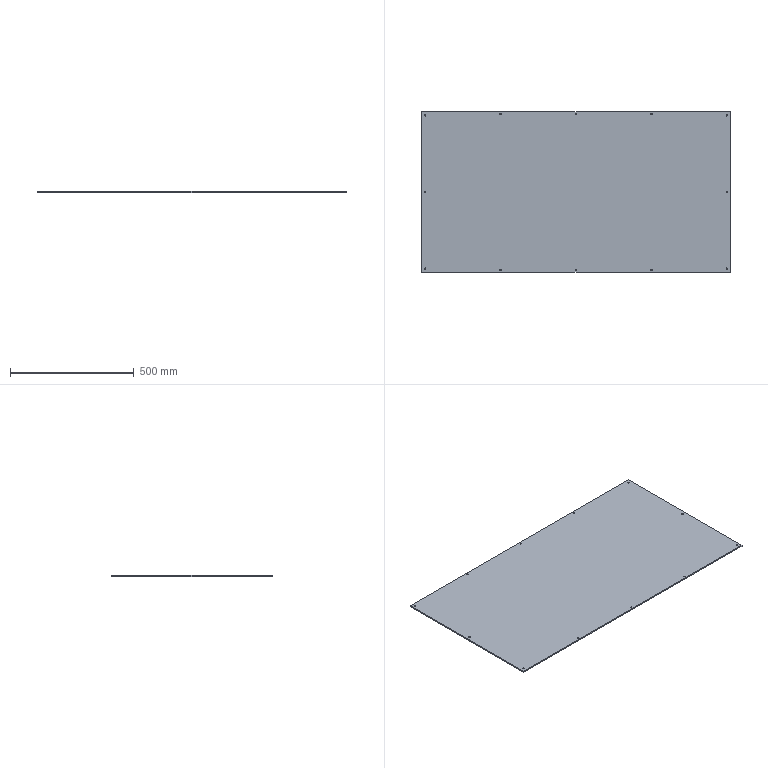Part | SolidWorks | features BaseBody 1 | 1 solid | 30 faces | box 1250 x 650 x 5 mm | volume 4061075 mm3 | cylinder 24 | plane 6 | commonest cylinder face diameters 5.5 x24
STEP:
#1=CARTESIAN_POINT('',(607.25,0.,-2.5));
#2=VERTEX_POINT('',#1);
#3=CARTESIAN_POINT('',(612.75,0.,-2.5));
#4=VERTEX_POINT('',#3);
#5=CARTESIAN_POINT('',(610.,0.,-2.5));
#6=DIRECTION('',(0.,0.,1.));
#7=DIRECTION('',(1.,0.,0.));
#8=AXIS2_PLACEMENT_3D('',#5,#6,#7);
#9=CIRCLE('',#8,2.75);
#10=EDGE_CURVE('',#2,#4,#9,.T.);
#11=ORIENTED_EDGE('',*,*,#10,.F.);
#12=CARTESIAN_POINT('',(607.25,0.,2.5));
#13=VERTEX_POINT('',#12);
#14=CARTESIAN_POINT('',(607.25,0.,2.5));
#15=DIRECTION('',(0.,0.,1.));
#16=VECTOR('',#15,1000.);
#17=LINE('',#14,#16);
#18=EDGE_CURVE('',#2,#13,#17,.T.);
#19=ORIENTED_EDGE('',*,*,#18,.T.);
#20=CARTESIAN_POINT('',(612.75,0.,2.5));
#21=VERTEX_POINT('',#20);
#22=CARTESIAN_POINT('',(610.,0.,2.5));
#23=DIRECTION('',(0.,0.,1.));
#24=DIRECTION('',(1.,0.,0.));
#25=AXIS2_PLACEMENT_3D('',#22,#23,#24);
#26=CIRCLE('',#25,2.75);
#27=EDGE_CURVE('',#13,#21,#26,.T.);
#28=ORIENTED_EDGE('',*,*,#27,.T.);
#29=CARTESIAN_POINT('',(612.75,0.,2.5));
#30=DIRECTION('',(0.,0.,1.));
#31=VECTOR('',#30,1000.);
#32=LINE('',#29,#31);
#33=EDGE_CURVE('',#4,#21,#32,.T.);
#34=ORIENTED_EDGE('',*,*,#33,.F.);
#35=EDGE_LOOP('',(#11,#19,#28,#34));
#36=FACE_OUTER_BOUND('',#35,.T.);
#37=CARTESIAN_POINT('',(610.,0.,2.5));
#38=DIRECTION('',(0.,0.,1.));
#39=DIRECTION('',(1.,0.,0.));
#40=AXIS2_PLACEMENT_3D('',#37,#38,#39);
#41=CYLINDRICAL_SURFACE('',#40,2.75);
#42=ADVANCED_FACE('',(#36),#41,.F.);
#43=CARTESIAN_POINT('',(607.25,-310.,-2.5));
#44=VERTEX_POINT('',#43);
#45=CARTESIAN_POINT('',(612.75,-310.,-2.5));
#46=VERTEX_POINT('',#45);
#47=CARTESIAN_POINT('',(610.,-310.,-2.5));
#48=DIRECTION('',(0.,0.,1.));
#49=DIRECTION('',(1.,0.,0.));
#50=AXIS2_PLACEMENT_3D('',#47,#48,#49);
#51=CIRCLE('',#50,2.75);
#52=EDGE_CURVE('',#44,#46,#51,.T.);
#53=ORIENTED_EDGE('',*,*,#52,.F.);
#54=CARTESIAN_POINT('',(607.25,-310.,2.5));
#55=VERTEX_POINT('',#54);
#56=CARTESIAN_POINT('',(607.25,-310.,2.5));
#57=DIRECTION('',(0.,0.,1.));
#58=VECTOR('',#57,1000.);
#59=LINE('',#56,#58);
#60=EDGE_CURVE('',#44,#55,#59,.T.);
#61=ORIENTED_EDGE('',*,*,#60,.T.);
#62=CARTESIAN_POINT('',(612.75,-310.,2.5));
#63=VERTEX_POINT('',#62);
#64=CARTESIAN_POINT('',(610.,-310.,2.5));
#65=DIRECTION('',(0.,0.,1.));
#66=DIRECTION('',(1.,0.,0.));
#67=AXIS2_PLACEMENT_3D('',#64,#65,#66);
#68=CIRCLE('',#67,2.75);
#69=EDGE_CURVE('',#55,#63,#68,.T.);
#70=ORIENTED_EDGE('',*,*,#69,.T.);
#71=CARTESIAN_POINT('',(612.75,-310.,2.5));
#72=DIRECTION('',(0.,0.,1.));
#73=VECTOR('',#72,1000.);
#74=LINE('',#71,#73);
#75=EDGE_CURVE('',#46,#63,#74,.T.);
#76=ORIENTED_EDGE('',*,*,#75,.F.);
#77=EDGE_LOOP('',(#53,#61,#70,#76));
#78=FACE_OUTER_BOUND('',#77,.T.);
#79=CARTESIAN_POINT('',(610.,-310.,2.5));
#80=DIRECTION('',(0.,0.,1.));
#81=DIRECTION('',(1.,0.,0.));
#82=AXIS2_PLACEMENT_3D('',#79,#80,#81);
#83=CYLINDRICAL_SURFACE('',#82,2.75);
#84=ADVANCED_FACE('',(#78),#83,.F.);
#85=CARTESIAN_POINT('',(607.25,310.,-2.5));
#86=VERTEX_POINT('',#85);
#87=CARTESIAN_POINT('',(612.75,310.,-2.5));
#88=VERTEX_POINT('',#87);
#89=CARTESIAN_POINT('',(610.,310.,-2.5));
#90=DIRECTION('',(0.,0.,1.));
#91=DIRECTION('',(1.,0.,0.));
#92=AXIS2_PLACEMENT_3D('',#89,#90,#91);
#93=CIRCLE('',#92,2.75);
#94=EDGE_CURVE('',#86,#88,#93,.T.);
#95=ORIENTED_EDGE('',*,*,#94,.F.);
#96=CARTESIAN_POINT('',(607.25,310.,2.5));
#97=VERTEX_POINT('',#96);
#98=CARTESIAN_POINT('',(607.25,310.,2.5));
#99=DIRECTION('',(0.,0.,1.));
#100=VECTOR('',#99,1000.);
#101=LINE('',#98,#100);
#102=EDGE_CURVE('',#86,#97,#101,.T.);
#103=ORIENTED_EDGE('',*,*,#102,.T.);
#104=CARTESIAN_POINT('',(612.75,310.,2.5));
#105=VERTEX_POINT('',#104);
#106=CARTESIAN_POINT('',(610.,310.,2.5));
#107=DIRECTION('',(0.,0.,1.));
#108=DIRECTION('',(1.,0.,0.));
#109=AXIS2_PLACEMENT_3D('',#106,#107,#108);
#110=CIRCLE('',#109,2.75);
#111=EDGE_CURVE('',#97,#105,#110,.T.);
#112=ORIENTED_EDGE('',*,*,#111,.T.);
#113=CARTESIAN_POINT('',(612.75,310.,2.5));
#114=DIRECTION('',(0.,0.,1.));
#115=VECTOR('',#114,1000.);
#116=LINE('',#113,#115);
#117=EDGE_CURVE('',#88,#105,#116,.T.);
#118=ORIENTED_EDGE('',*,*,#117,.F.);
#119=EDGE_LOOP('',(#95,#103,#112,#118));
#120=FACE_OUTER_BOUND('',#119,.T.);
#121=CARTESIAN_POINT('',(610.,310.,2.5));
#122=DIRECTION('',(0.,0.,1.));
#123=DIRECTION('',(1.,0.,0.));
#124=AXIS2_PLACEMENT_3D('',#121,#122,#123);
#125=CYLINDRICAL_SURFACE('',#124,2.75);
#126=ADVANCED_FACE('',(#120),#125,.F.);
#127=CARTESIAN_POINT('',(302.25,-316.,-2.5));
#128=VERTEX_POINT('',#127);
#129=CARTESIAN_POINT('',(307.75,-316.,-2.5));
#130=VERTEX_POINT('',#129);
#131=CARTESIAN_POINT('',(305.,-316.,-2.5));
#132=DIRECTION('',(0.,0.,1.));
#133=DIRECTION('',(1.,0.,0.));
#134=AXIS2_PLACEMENT_3D('',#131,#132,#133);
#135=CIRCLE('',#134,2.75);
#136=EDGE_CURVE('',#128,#130,#135,.T.);
#137=ORIENTED_EDGE('',*,*,#136,.F.);
#138=CARTESIAN_POINT('',(302.25,-316.,2.5));
#139=VERTEX_POINT('',#138);
#140=CARTESIAN_POINT('',(302.25,-316.,2.5));
#141=DIRECTION('',(0.,0.,1.));
#142=VECTOR('',#141,1000.);
#143=LINE('',#140,#142);
#144=EDGE_CURVE('',#128,#139,#143,.T.);
#145=ORIENTED_EDGE('',*,*,#144,.T.);
#146=CARTESIAN_POINT('',(307.75,-316.,2.5));
#147=VERTEX_POINT('',#146);
#148=CARTESIAN_POINT('',(305.,-316.,2.5));
#149=DIRECTION('',(0.,0.,1.));
#150=DIRECTION('',(1.,0.,0.));
#151=AXIS2_PLACEMENT_3D('',#148,#149,#150);
#152=CIRCLE('',#151,2.75);
#153=EDGE_CURVE('',#139,#147,#152,.T.);
#154=ORIENTED_EDGE('',*,*,#153,.T.);
#155=CARTESIAN_POINT('',(307.75,-316.,2.5));
#156=DIRECTION('',(0.,0.,1.));
#157=VECTOR('',#156,1000.);
#158=LINE('',#155,#157);
#159=EDGE_CURVE('',#130,#147,#158,.T.);
#160=ORIENTED_EDGE('',*,*,#159,.F.);
#161=EDGE_LOOP('',(#137,#145,#154,#160));
#162=FACE_OUTER_BOUND('',#161,.T.);
#163=CARTESIAN_POINT('',(305.,-316.,2.5));
#164=DIRECTION('',(0.,0.,1.));
#165=DIRECTION('',(1.,0.,0.));
#166=AXIS2_PLACEMENT_3D('',#163,#164,#165);
#167=CYLINDRICAL_SURFACE('',#166,2.75);
#168=ADVANCED_FACE('',(#162),#167,.F.);
#169=CARTESIAN_POINT('',(302.25,316.,-2.5));
#170=VERTEX_POINT('',#169);
#171=CARTESIAN_POINT('',(307.75,316.,-2.5));
#172=VERTEX_POINT('',#171);
#173=CARTESIAN_POINT('',(305.,316.,-2.5));
#174=DIRECTION('',(0.,0.,1.));
#175=DIRECTION('',(1.,0.,0.));
#176=AXIS2_PLACEMENT_3D('',#173,#174,#175);
#177=CIRCLE('',#176,2.75);
#178=EDGE_CURVE('',#170,#172,#177,.T.);
#179=ORIENTED_EDGE('',*,*,#178,.F.);
#180=CARTESIAN_POINT('',(302.25,316.,2.5));
#181=VERTEX_POINT('',#180);
#182=CARTESIAN_POINT('',(302.25,316.,2.5));
#183=DIRECTION('',(0.,0.,1.));
#184=VECTOR('',#183,1000.);
#185=LINE('',#182,#184);
#186=EDGE_CURVE('',#170,#181,#185,.T.);
#187=ORIENTED_EDGE('',*,*,#186,.T.);
#188=CARTESIAN_POINT('',(307.75,316.,2.5));
#189=VERTEX_POINT('',#188);
#190=CARTESIAN_POINT('',(305.,316.,2.5));
#191=DIRECTION('',(0.,0.,1.));
#192=DIRECTION('',(1.,0.,0.));
#193=AXIS2_PLACEMENT_3D('',#190,#191,#192);
#194=CIRCLE('',#193,2.75);
#195=EDGE_CURVE('',#181,#189,#194,.T.);
#196=ORIENTED_EDGE('',*,*,#195,.T.);
#197=CARTESIAN_POINT('',(307.75,316.,2.5));
#198=DIRECTION('',(0.,0.,1.));
#199=VECTOR('',#198,1000.);
#200=LINE('',#197,#199);
#201=EDGE_CURVE('',#172,#189,#200,.T.);
#202=ORIENTED_EDGE('',*,*,#201,.F.);
#203=EDGE_LOOP('',(#179,#187,#196,#202));
#204=FACE_OUTER_BOUND('',#203,.T.);
#205=CARTESIAN_POINT('',(305.,316.,2.5));
#206=DIRECTION('',(0.,0.,1.));
#207=DIRECTION('',(1.,0.,0.));
#208=AXIS2_PLACEMENT_3D('',#205,#206,#207);
#209=CYLINDRICAL_SURFACE('',#208,2.75);
#210=ADVANCED_FACE('',(#204),#209,.F.);
#211=CARTESIAN_POINT('',(-2.75,-316.,-2.5));
#212=VERTEX_POINT('',#211);
#213=CARTESIAN_POINT('',(2.75,-316.,-2.5));
#214=VERTEX_POINT('',#213);
#215=CARTESIAN_POINT('',(0.,-316.,-2.5));
#216=DIRECTION('',(0.,0.,1.));
#217=DIRECTION('',(1.,0.,0.));
#218=AXIS2_PLACEMENT_3D('',#215,#216,#217);
#219=CIRCLE('',#218,2.75);
#220=EDGE_CURVE('',#212,#214,#219,.T.);
#221=ORIENTED_EDGE('',*,*,#220,.F.);
#222=CARTESIAN_POINT('',(-2.75,-316.,2.5));
#223=VERTEX_POINT('',#222);
#224=CARTESIAN_POINT('',(-2.75,-316.,2.5));
#225=DIRECTION('',(0.,0.,1.));
#226=VECTOR('',#225,1000.);
#227=LINE('',#224,#226);
#228=EDGE_CURVE('',#212,#223,#227,.T.);
#229=ORIENTED_EDGE('',*,*,#228,.T.);
#230=CARTESIAN_POINT('',(2.75,-316.,2.5));
#231=VERTEX_POINT('',#230);
#232=CARTESIAN_POINT('',(0.,-316.,2.5));
#233=DIRECTION('',(0.,0.,1.));
#234=DIRECTION('',(1.,0.,0.));
#235=AXIS2_PLACEMENT_3D('',#232,#233,#234);
#236=CIRCLE('',#235,2.75);
#237=EDGE_CURVE('',#223,#231,#236,.T.);
#238=ORIENTED_EDGE('',*,*,#237,.T.);
#239=CARTESIAN_POINT('',(2.75,-316.,2.5));
#240=DIRECTION('',(0.,0.,1.));
#241=VECTOR('',#240,1000.);
#242=LINE('',#239,#241);
#243=EDGE_CURVE('',#214,#231,#242,.T.);
#244=ORIENTED_EDGE('',*,*,#243,.F.);
#245=EDGE_LOOP('',(#221,#229,#238,#244));
#246=FACE_OUTER_BOUND('',#245,.T.);
#247=CARTESIAN_POINT('',(0.,-316.,2.5));
#248=DIRECTION('',(0.,0.,1.));
#249=DIRECTION('',(1.,0.,0.));
#250=AXIS2_PLACEMENT_3D('',#247,#248,#249);
#251=CYLINDRICAL_SURFACE('',#250,2.75);
#252=ADVANCED_FACE('',(#246),#251,.F.);
#253=CARTESIAN_POINT('',(-2.75,316.,-2.5));
#254=VERTEX_POINT('',#253);
#255=CARTESIAN_POINT('',(2.75,316.,-2.5));
#256=VERTEX_POINT('',#255);
#257=CARTESIAN_POINT('',(0.,316.,-2.5));
#258=DIRECTION('',(0.,0.,1.));
#259=DIRECTION('',(1.,0.,0.));
#260=AXIS2_PLACEMENT_3D('',#257,#258,#259);
#261=CIRCLE('',#260,2.75);
#262=EDGE_CURVE('',#254,#256,#261,.T.);
#263=ORIENTED_EDGE('',*,*,#262,.F.);
#264=CARTESIAN_POINT('',(-2.75,316.,2.5));
#265=VERTEX_POINT('',#264);
#266=CARTESIAN_POINT('',(-2.75,316.,2.5));
#267=DIRECTION('',(0.,0.,1.));
#268=VECTOR('',#267,1000.);
#269=LINE('',#266,#268);
#270=EDGE_CURVE('',#254,#265,#269,.T.);
#271=ORIENTED_EDGE('',*,*,#270,.T.);
#272=CARTESIAN_POINT('',(2.75,316.,2.5));
#273=VERTEX_POINT('',#272);
#274=CARTESIAN_POINT('',(0.,316.,2.5));
#275=DIRECTION('',(0.,0.,1.));
#276=DIRECTION('',(1.,0.,0.));
#277=AXIS2_PLACEMENT_3D('',#274,#275,#276);
#278=CIRCLE('',#277,2.75);
#279=EDGE_CURVE('',#265,#273,#278,.T.);
#280=ORIENTED_EDGE('',*,*,#279,.T.);
#281=CARTESIAN_POINT('',(2.75,316.,2.5));
#282=DIRECTION('',(0.,0.,1.));
#283=VECTOR('',#282,1000.);
#284=LINE('',#281,#283);
#285=EDGE_CURVE('',#256,#273,#284,.T.);
#286=ORIENTED_EDGE('',*,*,#285,.F.);
#287=EDGE_LOOP('',(#263,#271,#280,#286));
#288=FACE_OUTER_BOUND('',#287,.T.);
#289=CARTESIAN_POINT('',(0.,316.,2.5));
#290=DIRECTION('',(0.,0.,1.));
#291=DIRECTION('',(1.,0.,0.));
#292=AXIS2_PLACEMENT_3D('',#289,#290,#291);
#293=CYLINDRICAL_SURFACE('',#292,2.75);
#294=ADVANCED_FACE('',(#288),#293,.F.);
#295=CARTESIAN_POINT('',(-307.75,-316.,-2.5));
#296=VERTEX_POINT('',#295);
#297=CARTESIAN_POINT('',(-302.25,-316.,-2.5));
#298=VERTEX_POINT('',#297);
#299=CARTESIAN_POINT('',(-305.,-316.,-2.5));
#300=DIRECTION('',(0.,0.,1.));
#301=DIRECTION('',(1.,0.,0.));
#302=AXIS2_PLACEMENT_3D('',#299,#300,#301);
#303=CIRCLE('',#302,2.75);
#304=EDGE_CURVE('',#296,#298,#303,.T.);
#305=ORIENTED_EDGE('',*,*,#304,.F.);
#306=CARTESIAN_POINT('',(-307.75,-316.,2.5));
#307=VERTEX_POINT('',#306);
#308=CARTESIAN_POINT('',(-307.75,-316.,2.5));
#309=DIRECTION('',(0.,0.,1.));
#310=VECTOR('',#309,1000.);
#311=LINE('',#308,#310);
#312=EDGE_CURVE('',#296,#307,#311,.T.);
#313=ORIENTED_EDGE('',*,*,#312,.T.);
#314=CARTESIAN_POINT('',(-302.25,-316.,2.5));
#315=VERTEX_POINT('',#314);
#316=CARTESIAN_POINT('',(-305.,-316.,2.5));
#317=DIRECTION('',(0.,0.,1.));
#318=DIRECTION('',(1.,0.,0.));
#319=AXIS2_PLACEMENT_3D('',#316,#317,#318);
#320=CIRCLE('',#319,2.75);
#321=EDGE_CURVE('',#307,#315,#320,.T.);
#322=ORIENTED_EDGE('',*,*,#321,.T.);
#323=CARTESIAN_POINT('',(-302.25,-316.,2.5));
#324=DIRECTION('',(0.,0.,1.));
#325=VECTOR('',#324,1000.);
#326=LINE('',#323,#325);
#327=EDGE_CURVE('',#298,#315,#326,.T.);
#328=ORIENTED_EDGE('',*,*,#327,.F.);
#329=EDGE_LOOP('',(#305,#313,#322,#328));
#330=FACE_OUTER_BOUND('',#329,.T.);
#331=CARTESIAN_POINT('',(-305.,-316.,2.5));
#332=DIRECTION('',(0.,0.,1.));
#333=DIRECTION('',(1.,0.,0.));
#334=AXIS2_PLACEMENT_3D('',#331,#332,#333);
#335=CYLINDRICAL_SURFACE('',#334,2.75);
#336=ADVANCED_FACE('',(#330),#335,.F.);
#337=CARTESIAN_POINT('',(-307.75,316.,-2.5));
#338=VERTEX_POINT('',#337);
#339=CARTESIAN_POINT('',(-302.25,316.,-2.5));
#340=VERTEX_POINT('',#339);
#341=CARTESIAN_POINT('',(-305.,316.,-2.5));
#342=DIRECTION('',(0.,0.,1.));
#343=DIRECTION('',(1.,0.,0.));
#344=AXIS2_PLACEMENT_3D('',#341,#342,#343);
#345=CIRCLE('',#344,2.75);
#346=EDGE_CURVE('',#338,#340,#345,.T.);
#347=ORIENTED_EDGE('',*,*,#346,.F.);
#348=CARTESIAN_POINT('',(-307.75,316.,2.5));
#349=VERTEX_POINT('',#348);
#350=CARTESIAN_POINT('',(-307.75,316.,2.5));
#351=DIRECTION('',(0.,0.,1.));
#352=VECTOR('',#351,1000.);
#353=LINE('',#350,#352);
#354=EDGE_CURVE('',#338,#349,#353,.T.);
#355=ORIENTED_EDGE('',*,*,#354,.T.);
#356=CARTESIAN_POINT('',(-302.25,316.,2.5));
#357=VERTEX_POINT('',#356);
#358=CARTESIAN_POINT('',(-305.,316.,2.5));
#359=DIRECTION('',(0.,0.,1.));
#360=DIRECTION('',(1.,0.,0.));
#361=AXIS2_PLACEMENT_3D('',#358,#359,#360);
#362=CIRCLE('',#361,2.75);
#363=EDGE_CURVE('',#349,#357,#362,.T.);
#364=ORIENTED_EDGE('',*,*,#363,.T.);
#365=CARTESIAN_POINT('',(-302.25,316.,2.5));
#366=DIRECTION('',(0.,0.,1.));
#367=VECTOR('',#366,1000.);
#368=LINE('',#365,#367);
#369=EDGE_CURVE('',#340,#357,#368,.T.);
#370=ORIENTED_EDGE('',*,*,#369,.F.);
#371=EDGE_LOOP('',(#347,#355,#364,#370));
#372=FACE_OUTER_BOUND('',#371,.T.);
#373=CARTESIAN_POINT('',(-305.,316.,2.5));
#374=DIRECTION('',(0.,0.,1.));
#375=DIRECTION('',(1.,0.,0.));
#376=AXIS2_PLACEMENT_3D('',#373,#374,#375);
#377=CYLINDRICAL_SURFACE('',#376,2.75);
#378=ADVANCED_FACE('',(#372),#377,.F.);
#379=CARTESIAN_POINT('',(-612.75,-310.,-2.5));
#380=VERTEX_POINT('',#379);
#381=CARTESIAN_POINT('',(-607.25,-310.,-2.5));
#382=VERTEX_POINT('',#381);
#383=CARTESIAN_POINT('',(-610.,-310.,-2.5));
#384=DIRECTION('',(0.,0.,1.));
#385=DIRECTION('',(1.,0.,0.));
#386=AXIS2_PLACEMENT_3D('',#383,#384,#385);
#387=CIRCLE('',#386,2.75);
#388=EDGE_CURVE('',#380,#382,#387,.T.);
#389=ORIENTED_EDGE('',*,*,#388,.F.);
#390=CARTESIAN_POINT('',(-612.75,-310.,2.5));
#391=VERTEX_POINT('',#390);
#392=CARTESIAN_POINT('',(-612.75,-310.,2.5));
#393=DIRECTION('',(0.,0.,1.));
#394=VECTOR('',#393,1000.);
#395=LINE('',#392,#394);
#396=EDGE_CURVE('',#380,#391,#395,.T.);
#397=ORIENTED_EDGE('',*,*,#396,.T.);
#398=CARTESIAN_POINT('',(-607.25,-310.,2.5));
#399=VERTEX_POINT('',#398);
#400=CARTESIAN_POINT('',(-610.,-310.,2.5));
#401=DIRECTION('',(0.,0.,1.));
#402=DIRECTION('',(1.,0.,0.));
#403=AXIS2_PLACEMENT_3D('',#400,#401,#402);
#404=CIRCLE('',#403,2.75);
#405=EDGE_CURVE('',#391,#399,#404,.T.);
#406=ORIENTED_EDGE('',*,*,#405,.T.);
#407=CARTESIAN_POINT('',(-607.25,-310.,2.5));
#408=DIRECTION('',(0.,0.,1.));
#409=VECTOR('',#408,1000.);
#410=LINE('',#407,#409);
#411=EDGE_CURVE('',#382,#399,#410,.T.);
#412=ORIENTED_EDGE('',*,*,#411,.F.);
#413=EDGE_LOOP('',(#389,#397,#406,#412));
#414=FACE_OUTER_BOUND('',#413,.T.);
#415=CARTESIAN_POINT('',(-610.,-310.,2.5));
#416=DIRECTION('',(0.,0.,1.));
#417=DIRECTION('',(1.,0.,0.));
#418=AXIS2_PLACEMENT_3D('',#415,#416,#417);
#419=CYLINDRICAL_SURFACE('',#418,2.75);
#420=ADVANCED_FACE('',(#414),#419,.F.);
#421=CARTESIAN_POINT('',(-612.75,0.,-2.5));
#422=VERTEX_POINT('',#421);
#423=CARTESIAN_POINT('',(-607.25,0.,-2.5));
#424=VERTEX_POINT('',#423);
#425=CARTESIAN_POINT('',(-610.,0.,-2.5));
#426=DIRECTION('',(0.,0.,1.));
#427=DIRECTION('',(1.,0.,0.));
#428=AXIS2_PLACEMENT_3D('',#425,#426,#427);
#429=CIRCLE('',#428,2.75);
#430=EDGE_CURVE('',#422,#424,#429,.T.);
#431=ORIENTED_EDGE('',*,*,#430,.F.);
#432=CARTESIAN_POINT('',(-612.75,0.,2.5));
#433=VERTEX_POINT('',#432);
#434=CARTESIAN_POINT('',(-612.75,0.,2.5));
#435=DIRECTION('',(0.,0.,1.));
#436=VECTOR('',#435,1000.);
#437=LINE('',#434,#436);
#438=EDGE_CURVE('',#422,#433,#437,.T.);
#439=ORIENTED_EDGE('',*,*,#438,.T.);
#440=CARTESIAN_POINT('',(-607.25,0.,2.5));
#441=VERTEX_POINT('',#440);
#442=CARTESIAN_POINT('',(-610.,0.,2.5));
#443=DIRECTION('',(0.,0.,1.));
#444=DIRECTION('',(1.,0.,0.));
#445=AXIS2_PLACEMENT_3D('',#442,#443,#444);
#446=CIRCLE('',#445,2.75);
#447=EDGE_CURVE('',#433,#441,#446,.T.);
#448=ORIENTED_EDGE('',*,*,#447,.T.);
#449=CARTESIAN_POINT('',(-607.25,0.,2.5));
#450=DIRECTION('',(0.,0.,1.));
#451=VECTOR('',#450,1000.);
#452=LINE('',#449,#451);
#453=EDGE_CURVE('',#424,#441,#452,.T.);
#454=ORIENTED_EDGE('',*,*,#453,.F.);
#455=EDGE_LOOP('',(#431,#439,#448,#454));
#456=FACE_OUTER_BOUND('',#455,.T.);
#457=CARTESIAN_POINT('',(-610.,0.,2.5));
#458=DIRECTION('',(0.,0.,1.));
#459=DIRECTION('',(1.,0.,0.));
#460=AXIS2_PLACEMENT_3D('',#457,#458,#459);
#461=CYLINDRICAL_SURFACE('',#460,2.75);
#462=ADVANCED_FACE('',(#456),#461,.F.);
#463=CARTESIAN_POINT('',(-612.75,310.,-2.5));
#464=VERTEX_POINT('',#463);
#465=CARTESIAN_POINT('',(-607.25,310.,-2.5));
#466=VERTEX_POINT('',#465);
#467=CARTESIAN_POINT('',(-610.,310.,-2.5));
#468=DIRECTION('',(0.,0.,1.));
#469=DIRECTION('',(1.,0.,0.));
#470=AXIS2_PLACEMENT_3D('',#467,#468,#469);
#471=CIRCLE('',#470,2.75);
#472=EDGE_CURVE('',#464,#466,#471,.T.);
#473=ORIENTED_EDGE('',*,*,#472,.F.);
#474=CARTESIAN_POINT('',(-612.75,310.,2.5));
#475=VERTEX_POINT('',#474);
#476=CARTESIAN_POINT('',(-612.75,310.,2.5));
#477=DIRECTION('',(0.,0.,1.));
#478=VECTOR('',#477,1000.);
#479=LINE('',#476,#478);
#480=EDGE_CURVE('',#464,#475,#479,.T.);
#481=ORIENTED_EDGE('',*,*,#480,.T.);
#482=CARTESIAN_POINT('',(-607.25,310.,2.5));
#483=VERTEX_POINT('',#482);
#484=CARTESIAN_POINT('',(-610.,310.,2.5));
#485=DIRECTION('',(0.,0.,1.));
#486=DIRECTION('',(1.,0.,0.));
#487=AXIS2_PLACEMENT_3D('',#484,#485,#486);
#488=CIRCLE('',#487,2.75);
#489=EDGE_CURVE('',#475,#483,#488,.T.);
#490=ORIENTED_EDGE('',*,*,#489,.T.);
#491=CARTESIAN_POINT('',(-607.25,310.,2.5));
#492=DIRECTION('',(0.,0.,1.));
#493=VECTOR('',#492,1000.);
#494=LINE('',#491,#493);
#495=EDGE_CURVE('',#466,#483,#494,.T.);
#496=ORIENTED_EDGE('',*,*,#495,.F.);
#497=EDGE_LOOP('',(#473,#481,#490,#496));
#498=FACE_OUTER_BOUND('',#497,.T.);
#499=CARTESIAN_POINT('',(-610.,310.,2.5));
#500=DIRECTION('',(0.,0.,1.));
#501=DIRECTION('',(1.,0.,0.));
#502=AXIS2_PLACEMENT_3D('',#499,#500,#501);
#503=CYLINDRICAL_SURFACE('',#502,2.75);
#504=ADVANCED_FACE('',(#498),#503,.F.);
#505=CARTESIAN_POINT('',(-610.,310.,-2.5));
#506=DIRECTION('',(0.,0.,1.));
#507=DIRECTION('',(1.,0.,0.));
#508=AXIS2_PLACEMENT_3D('',#505,#506,#507);
#509=CIRCLE('',#508,2.75);
#510=EDGE_CURVE('',#466,#464,#509,.T.);
#511=ORIENTED_EDGE('',*,*,#510,.T.);
#512=ORIENTED_EDGE('',*,*,#472,.T.);
#513=EDGE_LOOP('',(#511,#512));
#514=FACE_BOUND('',#513,.T.);
#515=CARTESIAN_POINT('',(-610.,0.,-2.5));
#516=DIRECTION('',(0.,0.,1.));
#517=DIRECTION('',(1.,0.,0.));
#518=AXIS2_PLACEMENT_3D('',#515,#516,#517);
#519=CIRCLE('',#518,2.75);
#520=EDGE_CURVE('',#424,#422,#519,.T.);
#521=ORIENTED_EDGE('',*,*,#520,.T.);
#522=ORIENTED_EDGE('',*,*,#430,.T.);
#523=EDGE_LOOP('',(#521,#522));
#524=FACE_BOUND('',#523,.T.);
#525=CARTESIAN_POINT('',(-610.,-310.,-2.5));
#526=DIRECTION('',(0.,0.,1.));
#527=DIRECTION('',(1.,0.,0.));
#528=AXIS2_PLACEMENT_3D('',#525,#526,#527);
#529=CIRCLE('',#528,2.75);
#530=EDGE_CURVE('',#382,#380,#529,.T.);
#531=ORIENTED_EDGE('',*,*,#530,.T.);
#532=ORIENTED_EDGE('',*,*,#388,.T.);
#533=EDGE_LOOP('',(#531,#532));
#534=FACE_BOUND('',#533,.T.);
#535=CARTESIAN_POINT('',(-305.,316.,-2.5));
#536=DIRECTION('',(0.,0.,1.));
#537=DIRECTION('',(1.,0.,0.));
#538=AXIS2_PLACEMENT_3D('',#535,#536,#537);
#539=CIRCLE('',#538,2.75);
#540=EDGE_CURVE('',#340,#338,#539,.T.);
#541=ORIENTED_EDGE('',*,*,#540,.T.);
#542=ORIENTED_EDGE('',*,*,#346,.T.);
#543=EDGE_LOOP('',(#541,#542));
#544=FACE_BOUND('',#543,.T.);
#545=CARTESIAN_POINT('',(-305.,-316.,-2.5));
#546=DIRECTION('',(0.,0.,1.));
#547=DIRECTION('',(1.,0.,0.));
#548=AXIS2_PLACEMENT_3D('',#545,#546,#547);
#549=CIRCLE('',#548,2.75);
#550=EDGE_CURVE('',#298,#296,#549,.T.);
#551=ORIENTED_EDGE('',*,*,#550,.T.);
#552=ORIENTED_EDGE('',*,*,#304,.T.);
#553=EDGE_LOOP('',(#551,#552));
#554=FACE_BOUND('',#553,.T.);
#555=CARTESIAN_POINT('',(0.,316.,-2.5));
#556=DIRECTION('',(0.,0.,1.));
#557=DIRECTION('',(1.,0.,0.));
#558=AXIS2_PLACEMENT_3D('',#555,#556,#557);
#559=CIRCLE('',#558,2.75);
#560=EDGE_CURVE('',#256,#254,#559,.T.);
#561=ORIENTED_EDGE('',*,*,#560,.T.);
#562=ORIENTED_EDGE('',*,*,#262,.T.);
#563=EDGE_LOOP('',(#561,#562));
#564=FACE_BOUND('',#563,.T.);
#565=CARTESIAN_POINT('',(0.,-316.,-2.5));
#566=DIRECTION('',(0.,0.,1.));
#567=DIRECTION('',(1.,0.,0.));
#568=AXIS2_PLACEMENT_3D('',#565,#566,#567);
#569=CIRCLE('',#568,2.75);
#570=EDGE_CURVE('',#214,#212,#569,.T.);
#571=ORIENTED_EDGE('',*,*,#570,.T.);
#572=ORIENTED_EDGE('',*,*,#220,.T.);
#573=EDGE_LOOP('',(#571,#572));
#574=FACE_BOUND('',#573,.T.);
#575=CARTESIAN_POINT('',(305.,316.,-2.5));
#576=DIRECTION('',(0.,0.,1.));
#577=DIRECTION('',(1.,0.,0.));
#578=AXIS2_PLACEMENT_3D('',#575,#576,#577);
#579=CIRCLE('',#578,2.75);
#580=EDGE_CURVE('',#172,#170,#579,.T.);
#581=ORIENTED_EDGE('',*,*,#580,.T.);
#582=ORIENTED_EDGE('',*,*,#178,.T.);
#583=EDGE_LOOP('',(#581,#582));
#584=FACE_BOUND('',#583,.T.);
#585=CARTESIAN_POINT('',(305.,-316.,-2.5));
#586=DIRECTION('',(0.,0.,1.));
#587=DIRECTION('',(1.,0.,0.));
#588=AXIS2_PLACEMENT_3D('',#585,#586,#587);
#589=CIRCLE('',#588,2.75);
#590=EDGE_CURVE('',#130,#128,#589,.T.);
#591=ORIENTED_EDGE('',*,*,#590,.T.);
#592=ORIENTED_EDGE('',*,*,#136,.T.);
#593=EDGE_LOOP('',(#591,#592));
#594=FACE_BOUND('',#593,.T.);
#595=CARTESIAN_POINT('',(610.,310.,-2.5));
#596=DIRECTION('',(0.,0.,1.));
#597=DIRECTION('',(1.,0.,0.));
#598=AXIS2_PLACEMENT_3D('',#595,#596,#597);
#599=CIRCLE('',#598,2.75);
#600=EDGE_CURVE('',#88,#86,#599,.T.);
#601=ORIENTED_EDGE('',*,*,#600,.T.);
#602=ORIENTED_EDGE('',*,*,#94,.T.);
#603=EDGE_LOOP('',(#601,#602));
#604=FACE_BOUND('',#603,.T.);
#605=CARTESIAN_POINT('',(610.,-310.,-2.5));
#606=DIRECTION('',(0.,0.,1.));
#607=DIRECTION('',(1.,0.,0.));
#608=AXIS2_PLACEMENT_3D('',#605,#606,#607);
#609=CIRCLE('',#608,2.75);
#610=EDGE_CURVE('',#46,#44,#609,.T.);
#611=ORIENTED_EDGE('',*,*,#610,.T.);
#612=ORIENTED_EDGE('',*,*,#52,.T.);
#613=EDGE_LOOP('',(#611,#612));
#614=FACE_BOUND('',#613,.T.);
#615=CARTESIAN_POINT('',(610.,0.,-2.5));
#616=DIRECTION('',(0.,0.,1.));
#617=DIRECTION('',(1.,0.,0.));
#618=AXIS2_PLACEMENT_3D('',#615,#616,#617);
#619=CIRCLE('',#618,2.75);
#620=EDGE_CURVE('',#4,#2,#619,.T.);
#621=ORIENTED_EDGE('',*,*,#620,.T.);
#622=ORIENTED_EDGE('',*,*,#10,.T.);
#623=EDGE_LOOP('',(#621,#622));
#624=FACE_BOUND('',#623,.T.);
#625=CARTESIAN_POINT('',(625.,-325.,-2.5));
#626=VERTEX_POINT('',#625);
#627=CARTESIAN_POINT('',(625.,325.,-2.5));
#628=VERTEX_POINT('',#627);
#629=CARTESIAN_POINT('',(625.,-325.,-2.5));
#630=DIRECTION('',(0.,1.,0.));
#631=VECTOR('',#630,1000.);
#632=LINE('',#629,#631);
#633=EDGE_CURVE('',#626,#628,#632,.T.);
#634=ORIENTED_EDGE('',*,*,#633,.F.);
#635=CARTESIAN_POINT('',(-625.,-325.,-2.5));
#636=VERTEX_POINT('',#635);
#637=CARTESIAN_POINT('',(-625.,-325.,-2.5));
#638=DIRECTION('',(1.,0.,0.));
#639=VECTOR('',#638,1000.);
#640=LINE('',#637,#639);
#641=EDGE_CURVE('',#636,#626,#640,.T.);
#642=ORIENTED_EDGE('',*,*,#641,.F.);
#643=CARTESIAN_POINT('',(-625.,325.,-2.5));
#644=VERTEX_POINT('',#643);
#645=CARTESIAN_POINT('',(-625.,-325.,-2.5));
#646=DIRECTION('',(0.,-1.,0.));
#647=VECTOR('',#646,1000.);
#648=LINE('',#645,#647);
#649=EDGE_CURVE('',#644,#636,#648,.T.);
#650=ORIENTED_EDGE('',*,*,#649,.F.);
#651=CARTESIAN_POINT('',(-625.,325.,-2.5));
#652=DIRECTION('',(-1.,0.,0.));
#653=VECTOR('',#652,1000.);
#654=LINE('',#651,#653);
#655=EDGE_CURVE('',#628,#644,#654,.T.);
#656=ORIENTED_EDGE('',*,*,#655,.F.);
#657=EDGE_LOOP('',(#634,#642,#650,#656));
#658=FACE_OUTER_BOUND('',#657,.T.);
#659=CARTESIAN_POINT('',(0.,0.,-2.5));
#660=DIRECTION('',(0.,0.,-1.));
#661=DIRECTION('',(0.,-1.,0.));
#662=AXIS2_PLACEMENT_3D('',#659,#660,#661);
#663=PLANE('',#662);
#664=ADVANCED_FACE('',(#514,#524,#534,#544,#554,#564,#574,#584,#594,#604,#614,#624,#658),#663,.T.);
#665=CARTESIAN_POINT('',(-610.,310.,2.5));
#666=DIRECTION('',(0.,0.,1.));
#667=DIRECTION('',(1.,0.,0.));
#668=AXIS2_PLACEMENT_3D('',#665,#666,#667);
#669=CIRCLE('',#668,2.75);
#670=EDGE_CURVE('',#483,#475,#669,.T.);
#671=ORIENTED_EDGE('',*,*,#670,.F.);
#672=ORIENTED_EDGE('',*,*,#489,.F.);
#673=EDGE_LOOP('',(#671,#672));
#674=FACE_BOUND('',#673,.T.);
#675=CARTESIAN_POINT('',(-610.,0.,2.5));
#676=DIRECTION('',(0.,0.,1.));
#677=DIRECTION('',(1.,0.,0.));
#678=AXIS2_PLACEMENT_3D('',#675,#676,#677);
#679=CIRCLE('',#678,2.75);
#680=EDGE_CURVE('',#441,#433,#679,.T.);
#681=ORIENTED_EDGE('',*,*,#680,.F.);
#682=ORIENTED_EDGE('',*,*,#447,.F.);
#683=EDGE_LOOP('',(#681,#682));
#684=FACE_BOUND('',#683,.T.);
#685=CARTESIAN_POINT('',(-610.,-310.,2.5));
#686=DIRECTION('',(0.,0.,1.));
#687=DIRECTION('',(1.,0.,0.));
#688=AXIS2_PLACEMENT_3D('',#685,#686,#687);
#689=CIRCLE('',#688,2.75);
#690=EDGE_CURVE('',#399,#391,#689,.T.);
#691=ORIENTED_EDGE('',*,*,#690,.F.);
#692=ORIENTED_EDGE('',*,*,#405,.F.);
#693=EDGE_LOOP('',(#691,#692));
#694=FACE_BOUND('',#693,.T.);
#695=CARTESIAN_POINT('',(-305.,316.,2.5));
#696=DIRECTION('',(0.,0.,1.));
#697=DIRECTION('',(1.,0.,0.));
#698=AXIS2_PLACEMENT_3D('',#695,#696,#697);
#699=CIRCLE('',#698,2.75);
#700=EDGE_CURVE('',#357,#349,#699,.T.);
#701=ORIENTED_EDGE('',*,*,#700,.F.);
#702=ORIENTED_EDGE('',*,*,#363,.F.);
#703=EDGE_LOOP('',(#701,#702));
#704=FACE_BOUND('',#703,.T.);
#705=CARTESIAN_POINT('',(-305.,-316.,2.5));
#706=DIRECTION('',(0.,0.,1.));
#707=DIRECTION('',(1.,0.,0.));
#708=AXIS2_PLACEMENT_3D('',#705,#706,#707);
#709=CIRCLE('',#708,2.75);
#710=EDGE_CURVE('',#315,#307,#709,.T.);
#711=ORIENTED_EDGE('',*,*,#710,.F.);
#712=ORIENTED_EDGE('',*,*,#321,.F.);
#713=EDGE_LOOP('',(#711,#712));
#714=FACE_BOUND('',#713,.T.);
#715=CARTESIAN_POINT('',(0.,316.,2.5));
#716=DIRECTION('',(0.,0.,1.));
#717=DIRECTION('',(1.,0.,0.));
#718=AXIS2_PLACEMENT_3D('',#715,#716,#717);
#719=CIRCLE('',#718,2.75);
#720=EDGE_CURVE('',#273,#265,#719,.T.);
#721=ORIENTED_EDGE('',*,*,#720,.F.);
#722=ORIENTED_EDGE('',*,*,#279,.F.);
#723=EDGE_LOOP('',(#721,#722));
#724=FACE_BOUND('',#723,.T.);
#725=CARTESIAN_POINT('',(0.,-316.,2.5));
#726=DIRECTION('',(0.,0.,1.));
#727=DIRECTION('',(1.,0.,0.));
#728=AXIS2_PLACEMENT_3D('',#725,#726,#727);
#729=CIRCLE('',#728,2.75);
#730=EDGE_CURVE('',#231,#223,#729,.T.);
#731=ORIENTED_EDGE('',*,*,#730,.F.);
#732=ORIENTED_EDGE('',*,*,#237,.F.);
#733=EDGE_LOOP('',(#731,#732));
#734=FACE_BOUND('',#733,.T.);
#735=CARTESIAN_POINT('',(305.,316.,2.5));
#736=DIRECTION('',(0.,0.,1.));
#737=DIRECTION('',(1.,0.,0.));
#738=AXIS2_PLACEMENT_3D('',#735,#736,#737);
#739=CIRCLE('',#738,2.75);
#740=EDGE_CURVE('',#189,#181,#739,.T.);
#741=ORIENTED_EDGE('',*,*,#740,.F.);
#742=ORIENTED_EDGE('',*,*,#195,.F.);
#743=EDGE_LOOP('',(#741,#742));
#744=FACE_BOUND('',#743,.T.);
#745=CARTESIAN_POINT('',(305.,-316.,2.5));
#746=DIRECTION('',(0.,0.,1.));
#747=DIRECTION('',(1.,0.,0.));
#748=AXIS2_PLACEMENT_3D('',#745,#746,#747);
#749=CIRCLE('',#748,2.75);
#750=EDGE_CURVE('',#147,#139,#749,.T.);
#751=ORIENTED_EDGE('',*,*,#750,.F.);
#752=ORIENTED_EDGE('',*,*,#153,.F.);
#753=EDGE_LOOP('',(#751,#752));
#754=FACE_BOUND('',#753,.T.);
#755=CARTESIAN_POINT('',(610.,310.,2.5));
#756=DIRECTION('',(0.,0.,1.));
#757=DIRECTION('',(1.,0.,0.));
#758=AXIS2_PLACEMENT_3D('',#755,#756,#757);
#759=CIRCLE('',#758,2.75);
#760=EDGE_CURVE('',#105,#97,#759,.T.);
#761=ORIENTED_EDGE('',*,*,#760,.F.);
#762=ORIENTED_EDGE('',*,*,#111,.F.);
#763=EDGE_LOOP('',(#761,#762));
#764=FACE_BOUND('',#763,.T.);
#765=CARTESIAN_POINT('',(610.,-310.,2.5));
#766=DIRECTION('',(0.,0.,1.));
#767=DIRECTION('',(1.,0.,0.));
#768=AXIS2_PLACEMENT_3D('',#765,#766,#767);
#769=CIRCLE('',#768,2.75);
#770=EDGE_CURVE('',#63,#55,#769,.T.);
#771=ORIENTED_EDGE('',*,*,#770,.F.);
#772=ORIENTED_EDGE('',*,*,#69,.F.);
#773=EDGE_LOOP('',(#771,#772));
#774=FACE_BOUND('',#773,.T.);
#775=CARTESIAN_POINT('',(610.,0.,2.5));
#776=DIRECTION('',(0.,0.,1.));
#777=DIRECTION('',(1.,0.,0.));
#778=AXIS2_PLACEMENT_3D('',#775,#776,#777);
#779=CIRCLE('',#778,2.75);
#780=EDGE_CURVE('',#21,#13,#779,.T.);
#781=ORIENTED_EDGE('',*,*,#780,.F.);
#782=ORIENTED_EDGE('',*,*,#27,.F.);
#783=EDGE_LOOP('',(#781,#782));
#784=FACE_BOUND('',#783,.T.);
#785=CARTESIAN_POINT('',(625.,-325.,2.5));
#786=VERTEX_POINT('',#785);
#787=CARTESIAN_POINT('',(625.,325.,2.5));
#788=VERTEX_POINT('',#787);
#789=CARTESIAN_POINT('',(625.,-325.,2.5));
#790=DIRECTION('',(0.,1.,0.));
#791=VECTOR('',#790,1000.);
#792=LINE('',#789,#791);
#793=EDGE_CURVE('',#786,#788,#792,.T.);
#794=ORIENTED_EDGE('',*,*,#793,.T.);
#795=CARTESIAN_POINT('',(-625.,325.,2.5));
#796=VERTEX_POINT('',#795);
#797=CARTESIAN_POINT('',(-625.,325.,2.5));
#798=DIRECTION('',(-1.,0.,0.));
#799=VECTOR('',#798,1000.);
#800=LINE('',#797,#799);
#801=EDGE_CURVE('',#788,#796,#800,.T.);
#802=ORIENTED_EDGE('',*,*,#801,.T.);
#803=CARTESIAN_POINT('',(-625.,-325.,2.5));
#804=VERTEX_POINT('',#803);
#805=CARTESIAN_POINT('',(-625.,-325.,2.5));
#806=DIRECTION('',(0.,-1.,0.));
#807=VECTOR('',#806,1000.);
#808=LINE('',#805,#807);
#809=EDGE_CURVE('',#796,#804,#808,.T.);
#810=ORIENTED_EDGE('',*,*,#809,.T.);
#811=CARTESIAN_POINT('',(-625.,-325.,2.5));
#812=DIRECTION('',(1.,0.,0.));
#813=VECTOR('',#812,1000.);
#814=LINE('',#811,#813);
#815=EDGE_CURVE('',#804,#786,#814,.T.);
#816=ORIENTED_EDGE('',*,*,#815,.T.);
#817=EDGE_LOOP('',(#794,#802,#810,#816));
#818=FACE_OUTER_BOUND('',#817,.T.);
#819=CARTESIAN_POINT('',(0.,0.,2.5));
#820=DIRECTION('',(0.,0.,-1.));
#821=DIRECTION('',(0.,-1.,0.));
#822=AXIS2_PLACEMENT_3D('',#819,#820,#821);
#823=PLANE('',#822);
#824=ADVANCED_FACE('',(#674,#684,#694,#704,#714,#724,#734,#744,#754,#764,#774,#784,#818),#823,.F.);
#825=ORIENTED_EDGE('',*,*,#641,.T.);
#826=CARTESIAN_POINT('',(625.,-325.,2.5));
#827=DIRECTION('',(0.,0.,-1.));
#828=VECTOR('',#827,1000.);
#829=LINE('',#826,#828);
#830=EDGE_CURVE('',#786,#626,#829,.T.);
#831=ORIENTED_EDGE('',*,*,#830,.F.);
#832=ORIENTED_EDGE('',*,*,#815,.F.);
#833=CARTESIAN_POINT('',(-625.,-325.,2.5));
#834=DIRECTION('',(0.,0.,-1.));
#835=VECTOR('',#834,1000.);
#836=LINE('',#833,#835);
#837=EDGE_CURVE('',#804,#636,#836,.T.);
#838=ORIENTED_EDGE('',*,*,#837,.T.);
#839=EDGE_LOOP('',(#825,#831,#832,#838));
#840=FACE_OUTER_BOUND('',#839,.T.);
#841=CARTESIAN_POINT('',(-625.,-325.,2.5));
#842=DIRECTION('',(0.,1.,0.));
#843=DIRECTION('',(1.,0.,0.));
#844=AXIS2_PLACEMENT_3D('',#841,#842,#843);
#845=PLANE('',#844);
#846=ADVANCED_FACE('',(#840),#845,.F.);
#847=ORIENTED_EDGE('',*,*,#649,.T.);
#848=ORIENTED_EDGE('',*,*,#837,.F.);
#849=ORIENTED_EDGE('',*,*,#809,.F.);
#850=CARTESIAN_POINT('',(-625.,325.,2.5));
#851=DIRECTION('',(0.,0.,-1.));
#852=VECTOR('',#851,1000.);
#853=LINE('',#850,#852);
#854=EDGE_CURVE('',#796,#644,#853,.T.);
#855=ORIENTED_EDGE('',*,*,#854,.T.);
#856=EDGE_LOOP('',(#847,#848,#849,#855));
#857=FACE_OUTER_BOUND('',#856,.T.);
#858=CARTESIAN_POINT('',(-625.,-325.,2.5));
#859=DIRECTION('',(1.,0.,0.));
#860=DIRECTION('',(0.,1.,0.));
#861=AXIS2_PLACEMENT_3D('',#858,#859,#860);
#862=PLANE('',#861);
#863=ADVANCED_FACE('',(#857),#862,.F.);
#864=ORIENTED_EDGE('',*,*,#655,.T.);
#865=ORIENTED_EDGE('',*,*,#854,.F.);
#866=ORIENTED_EDGE('',*,*,#801,.F.);
#867=CARTESIAN_POINT('',(625.,325.,2.5));
#868=DIRECTION('',(0.,0.,-1.));
#869=VECTOR('',#868,1000.);
#870=LINE('',#867,#869);
#871=EDGE_CURVE('',#788,#628,#870,.T.);
#872=ORIENTED_EDGE('',*,*,#871,.T.);
#873=EDGE_LOOP('',(#864,#865,#866,#872));
#874=FACE_OUTER_BOUND('',#873,.T.);
#875=CARTESIAN_POINT('',(-625.,325.,2.5));
#876=DIRECTION('',(0.,-1.,0.));
#877=DIRECTION('',(0.,0.,-1.));
#878=AXIS2_PLACEMENT_3D('',#875,#876,#877);
#879=PLANE('',#878);
#880=ADVANCED_FACE('',(#874),#879,.F.);
#881=ORIENTED_EDGE('',*,*,#633,.T.);
#882=ORIENTED_EDGE('',*,*,#871,.F.);
#883=ORIENTED_EDGE('',*,*,#793,.F.);
#884=ORIENTED_EDGE('',*,*,#830,.T.);
#885=EDGE_LOOP('',(#881,#882,#883,#884));
#886=FACE_OUTER_BOUND('',#885,.T.);
#887=CARTESIAN_POINT('',(625.,-325.,2.5));
#888=DIRECTION('',(-1.,0.,0.));
#889=DIRECTION('',(0.,0.,1.));
#890=AXIS2_PLACEMENT_3D('',#887,#888,#889);
#891=PLANE('',#890);
#892=ADVANCED_FACE('',(#886),#891,.F.);
#893=ORIENTED_EDGE('',*,*,#480,.F.);
#894=ORIENTED_EDGE('',*,*,#510,.F.);
#895=ORIENTED_EDGE('',*,*,#495,.T.);
#896=ORIENTED_EDGE('',*,*,#670,.T.);
#897=EDGE_LOOP('',(#893,#894,#895,#896));
#898=FACE_OUTER_BOUND('',#897,.T.);
#899=CARTESIAN_POINT('',(-610.,310.,2.5));
#900=DIRECTION('',(0.,0.,1.));
#901=DIRECTION('',(1.,0.,0.));
#902=AXIS2_PLACEMENT_3D('',#899,#900,#901);
#903=CYLINDRICAL_SURFACE('',#902,2.75);
#904=ADVANCED_FACE('',(#898),#903,.F.);
#905=ORIENTED_EDGE('',*,*,#438,.F.);
#906=ORIENTED_EDGE('',*,*,#520,.F.);
#907=ORIENTED_EDGE('',*,*,#453,.T.);
#908=ORIENTED_EDGE('',*,*,#680,.T.);
#909=EDGE_LOOP('',(#905,#906,#907,#908));
#910=FACE_OUTER_BOUND('',#909,.T.);
#911=CARTESIAN_POINT('',(-610.,0.,2.5));
#912=DIRECTION('',(0.,0.,1.));
#913=DIRECTION('',(1.,0.,0.));
#914=AXIS2_PLACEMENT_3D('',#911,#912,#913);
#915=CYLINDRICAL_SURFACE('',#914,2.75);
#916=ADVANCED_FACE('',(#910),#915,.F.);
#917=ORIENTED_EDGE('',*,*,#396,.F.);
#918=ORIENTED_EDGE('',*,*,#530,.F.);
#919=ORIENTED_EDGE('',*,*,#411,.T.);
#920=ORIENTED_EDGE('',*,*,#690,.T.);
#921=EDGE_LOOP('',(#917,#918,#919,#920));
#922=FACE_OUTER_BOUND('',#921,.T.);
#923=CARTESIAN_POINT('',(-610.,-310.,2.5));
#924=DIRECTION('',(0.,0.,1.));
#925=DIRECTION('',(1.,0.,0.));
#926=AXIS2_PLACEMENT_3D('',#923,#924,#925);
#927=CYLINDRICAL_SURFACE('',#926,2.75);
#928=ADVANCED_FACE('',(#922),#927,.F.);
#929=ORIENTED_EDGE('',*,*,#354,.F.);
#930=ORIENTED_EDGE('',*,*,#540,.F.);
#931=ORIENTED_EDGE('',*,*,#369,.T.);
#932=ORIENTED_EDGE('',*,*,#700,.T.);
#933=EDGE_LOOP('',(#929,#930,#931,#932));
#934=FACE_OUTER_BOUND('',#933,.T.);
#935=CARTESIAN_POINT('',(-305.,316.,2.5));
#936=DIRECTION('',(0.,0.,1.));
#937=DIRECTION('',(1.,0.,0.));
#938=AXIS2_PLACEMENT_3D('',#935,#936,#937);
#939=CYLINDRICAL_SURFACE('',#938,2.75);
#940=ADVANCED_FACE('',(#934),#939,.F.);
#941=ORIENTED_EDGE('',*,*,#312,.F.);
#942=ORIENTED_EDGE('',*,*,#550,.F.);
#943=ORIENTED_EDGE('',*,*,#327,.T.);
#944=ORIENTED_EDGE('',*,*,#710,.T.);
#945=EDGE_LOOP('',(#941,#942,#943,#944));
#946=FACE_OUTER_BOUND('',#945,.T.);
#947=CARTESIAN_POINT('',(-305.,-316.,2.5));
#948=DIRECTION('',(0.,0.,1.));
#949=DIRECTION('',(1.,0.,0.));
#950=AXIS2_PLACEMENT_3D('',#947,#948,#949);
#951=CYLINDRICAL_SURFACE('',#950,2.75);
#952=ADVANCED_FACE('',(#946),#951,.F.);
#953=ORIENTED_EDGE('',*,*,#270,.F.);
#954=ORIENTED_EDGE('',*,*,#560,.F.);
#955=ORIENTED_EDGE('',*,*,#285,.T.);
#956=ORIENTED_EDGE('',*,*,#720,.T.);
#957=EDGE_LOOP('',(#953,#954,#955,#956));
#958=FACE_OUTER_BOUND('',#957,.T.);
#959=CARTESIAN_POINT('',(0.,316.,2.5));
#960=DIRECTION('',(0.,0.,1.));
#961=DIRECTION('',(1.,0.,0.));
#962=AXIS2_PLACEMENT_3D('',#959,#960,#961);
#963=CYLINDRICAL_SURFACE('',#962,2.75);
#964=ADVANCED_FACE('',(#958),#963,.F.);
#965=ORIENTED_EDGE('',*,*,#228,.F.);
#966=ORIENTED_EDGE('',*,*,#570,.F.);
#967=ORIENTED_EDGE('',*,*,#243,.T.);
#968=ORIENTED_EDGE('',*,*,#730,.T.);
#969=EDGE_LOOP('',(#965,#966,#967,#968));
#970=FACE_OUTER_BOUND('',#969,.T.);
#971=CARTESIAN_POINT('',(0.,-316.,2.5));
#972=DIRECTION('',(0.,0.,1.));
#973=DIRECTION('',(1.,0.,0.));
#974=AXIS2_PLACEMENT_3D('',#971,#972,#973);
#975=CYLINDRICAL_SURFACE('',#974,2.75);
#976=ADVANCED_FACE('',(#970),#975,.F.);
#977=ORIENTED_EDGE('',*,*,#186,.F.);
#978=ORIENTED_EDGE('',*,*,#580,.F.);
#979=ORIENTED_EDGE('',*,*,#201,.T.);
#980=ORIENTED_EDGE('',*,*,#740,.T.);
#981=EDGE_LOOP('',(#977,#978,#979,#980));
#982=FACE_OUTER_BOUND('',#981,.T.);
#983=CARTESIAN_POINT('',(305.,316.,2.5));
#984=DIRECTION('',(0.,0.,1.));
#985=DIRECTION('',(1.,0.,0.));
#986=AXIS2_PLACEMENT_3D('',#983,#984,#985);
#987=CYLINDRICAL_SURFACE('',#986,2.75);
#988=ADVANCED_FACE('',(#982),#987,.F.);
#989=ORIENTED_EDGE('',*,*,#144,.F.);
#990=ORIENTED_EDGE('',*,*,#590,.F.);
#991=ORIENTED_EDGE('',*,*,#159,.T.);
#992=ORIENTED_EDGE('',*,*,#750,.T.);
#993=EDGE_LOOP('',(#989,#990,#991,#992));
#994=FACE_OUTER_BOUND('',#993,.T.);
#995=CARTESIAN_POINT('',(305.,-316.,2.5));
#996=DIRECTION('',(0.,0.,1.));
#997=DIRECTION('',(1.,0.,0.));
#998=AXIS2_PLACEMENT_3D('',#995,#996,#997);
#999=CYLINDRICAL_SURFACE('',#998,2.75);
#1000=ADVANCED_FACE('',(#994),#999,.F.);
#1001=ORIENTED_EDGE('',*,*,#102,.F.);
#1002=ORIENTED_EDGE('',*,*,#600,.F.);
#1003=ORIENTED_EDGE('',*,*,#117,.T.);
#1004=ORIENTED_EDGE('',*,*,#760,.T.);
#1005=EDGE_LOOP('',(#1001,#1002,#1003,#1004));
#1006=FACE_OUTER_BOUND('',#1005,.T.);
#1007=CARTESIAN_POINT('',(610.,310.,2.5));
#1008=DIRECTION('',(0.,0.,1.));
#1009=DIRECTION('',(1.,0.,0.));
#1010=AXIS2_PLACEMENT_3D('',#1007,#1008,#1009);
#1011=CYLINDRICAL_SURFACE('',#1010,2.75);
#1012=ADVANCED_FACE('',(#1006),#1011,.F.);
#1013=ORIENTED_EDGE('',*,*,#60,.F.);
#1014=ORIENTED_EDGE('',*,*,#610,.F.);
#1015=ORIENTED_EDGE('',*,*,#75,.T.);
#1016=ORIENTED_EDGE('',*,*,#770,.T.);
#1017=EDGE_LOOP('',(#1013,#1014,#1015,#1016));
#1018=FACE_OUTER_BOUND('',#1017,.T.);
#1019=CARTESIAN_POINT('',(610.,-310.,2.5));
#1020=DIRECTION('',(0.,0.,1.));
#1021=DIRECTION('',(1.,0.,0.));
#1022=AXIS2_PLACEMENT_3D('',#1019,#1020,#1021);
#1023=CYLINDRICAL_SURFACE('',#1022,2.75);
#1024=ADVANCED_FACE('',(#1018),#1023,.F.);
#1025=ORIENTED_EDGE('',*,*,#18,.F.);
#1026=ORIENTED_EDGE('',*,*,#620,.F.);
#1027=ORIENTED_EDGE('',*,*,#33,.T.);
#1028=ORIENTED_EDGE('',*,*,#780,.T.);
#1029=EDGE_LOOP('',(#1025,#1026,#1027,#1028));
#1030=FACE_OUTER_BOUND('',#1029,.T.);
#1031=CARTESIAN_POINT('',(610.,0.,2.5));
#1032=DIRECTION('',(0.,0.,1.));
#1033=DIRECTION('',(1.,0.,0.));
#1034=AXIS2_PLACEMENT_3D('',#1031,#1032,#1033);
#1035=CYLINDRICAL_SURFACE('',#1034,2.75);
#1036=ADVANCED_FACE('',(#1030),#1035,.F.);
#1037=CLOSED_SHELL('',(#42,#84,#126,#168,#210,#252,#294,#336,#378,#420,#462,#504,#664,#824,#846,#863,#880,#892,#904,#916,#928,#940,#952,#964,#976,#988,#1000,#1012,#1024,#1036));
#1038=MANIFOLD_SOLID_BREP('',#1037);
#1039=CARTESIAN_POINT('',(0.,0.,0.));
#1040=DIRECTION('',(0.,0.,1.));
#1041=DIRECTION('',(1.,0.,0.));
#1042=AXIS2_PLACEMENT_3D('',#1039,#1040,#1041);
#1043=(LENGTH_UNIT()NAMED_UNIT(*)SI_UNIT(.MILLI.,.METRE.));
#1044=UNCERTAINTY_MEASURE_WITH_UNIT(LENGTH_MEASURE(0.00001),#1043,'','');
#1045=(NAMED_UNIT(*)PLANE_ANGLE_UNIT()SI_UNIT($,.RADIAN.));
#1046=(NAMED_UNIT(*)SI_UNIT($,.STERADIAN.)SOLID_ANGLE_UNIT());
#1047=(GEOMETRIC_REPRESENTATION_CONTEXT(3)GLOBAL_UNCERTAINTY_ASSIGNED_CONTEXT((#1044))GLOBAL_UNIT_ASSIGNED_CONTEXT((#1043,#1045,#1046))REPRESENTATION_CONTEXT('',''));
#1048=ADVANCED_BREP_SHAPE_REPRESENTATION('',(#1038,#1042),#1047);